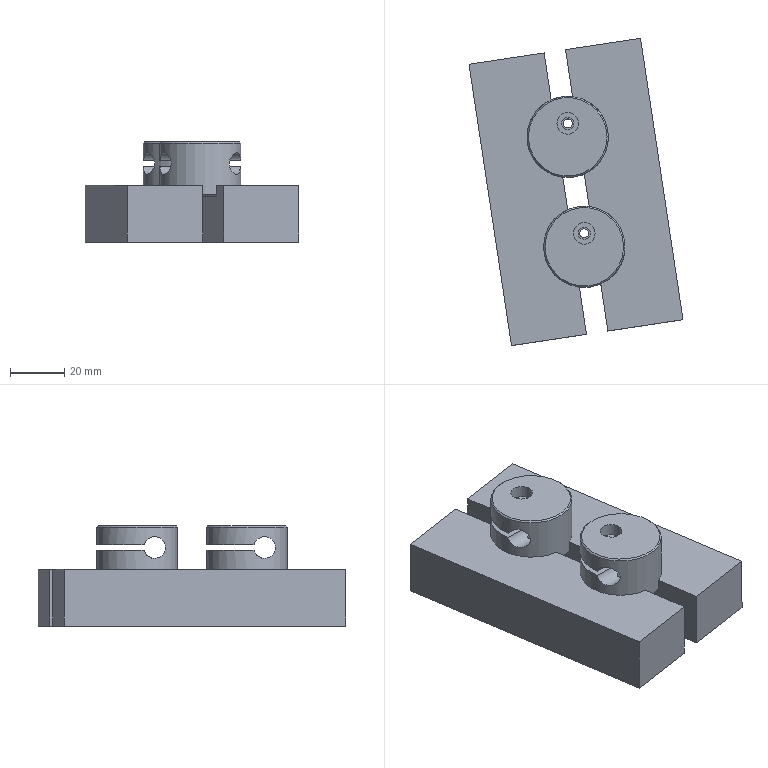CAM job | NX | 3-axis milling, drilling | part box 78.946 x 113.372 x 37 mm
Tools:
number,name,description,diameter,corner_radius,flute_length,length,flutes
3,D3,平底铣刀-粗,3.0,0.0,20.0,75.0,2
4,D4,平底铣刀-粗,4.0,0.0,25.0,75.0,2
8,D8,平底铣刀-粗,8.0,0.0,30.0,75.0,2
9,D10,平底铣刀-粗,10.0,0.0,35.0,75.0,2
10,D10-J,平底铣刀-精,10.0,0.0,35.0,75.0,2
1,D80R0.8飞刀,圆鼻刀-粗,80.0,0.8,50.0,75.0,2
2,D6倒角刀,倒角刀,6.0,0.0,3.0,25.0,2
20,M3X0.5,丝锥,2.5,0.0,35.0,50.0,2
21,M4X0.7,丝锥,3.3,0.0,35.0,50.0,2
12,ZT2.5,钻头,2.5,0.0,35.0,50.0,2
13,钻头3.3,Twist Drill 3.3 mm,3.3,0.0,35.0,35.008,2
Operations:
program,operation,operation_type,tool,method,geometry_group,spindle_rpm,surface_speed,feed_per_tooth,feed_cut,feed_plunge,cut_length_mm,path_length_mm,cut_time_min,machine_time_min
A,顶面,FaceMilling,D80R0.8飞刀,侧刃精光-切深K-步距G,W-A,4000.0,1005.31,0.125,1000.0,100.0,165.0,201.0,0.165,0.1686
A,动态开粗D8_COPY,CavityMilling,D8,动态开粗-切深K-步距K,W-A,8000.0,201.056,0.2188,3500.0,100.0,5250.862,5356.356,1.5,1.511
A,打点-深0.8,Operation,D6倒角刀,NONE,W-A,8000.0,150.796,0.0312,500.0,90.0,21.6,201.996,0.0432,0.0612
A,通孔-M3螺纹底孔,Operation,ZT2.5,NONE,W-A,3000.0,23.562,0.05,300.0,90.0,93.0,301.446,0.31,0.3308
A,盲锥孔-M3螺纹底孔,Operation,ZT2.5,NONE,W-A,3000.0,23.562,0.0167,100.0,90.0,64.0,234.601,0.64,0.6571
A,通孔-M4螺纹底孔,Operation,钻头3.3,NONE,W-A,3000.0,31.102,0.05,300.0,90.0,48.0,178.012,0.16,0.173
A,钻倒角_1,Operation,D6倒角刀,METHOD,W-A,8000.0,150.796,0.0312,500.0,0.0,47.5,272.832,0.095,0.1175
A,钻倒角_2,Operation,D6倒角刀,METHOD,W-A,8000.0,150.796,0.0312,500.0,0.0,10.4,104.91,0.0208,0.0303
A,底壁铣倒角_COPY,VolumeBased25DMillingOperation,D6倒角刀,爬面_倒角-切深0-步距G,W-A,6500.0,122.519,0.1154,1500.0,100.0,211.461,346.764,0.141,0.1545
A,盲锥孔-攻牙M3,Operation,M3X0.5,METHOD,W-A,1000.0,7.854,0.0003,0.5,90.0,48.0,202.601,96.0,96.016
A,通孔-攻牙M3,Operation,M3X0.5,METHOD,W-A,800.0,6.283,0.0003,0.5,90.0,78.0,271.446,156.0,156.019
A,通孔-攻牙M4,Operation,M4X0.7,METHOD,W-A,600.0,6.22,0.0006,0.7,90.0,30.0,142.012,42.857,42.868
A,外形半精_2,VolumeBased25DMillingOperation,D10-J,METHOD,W-A,8000.0,251.327,0.0625,1000.0,100.0,522.631,884.972,0.5226,0.5589
B,面铣自动飞面开粗一刀_COPY,FaceMilling,D80R0.8飞刀,分层开粗-切深K-步距G,W-B,4500.0,890.615,0.3333,3000.0,100.0,1917.474,3709.517,0.6392,0.8184
B,面铣自动飞面精光一刀_COPY,FaceMilling,D80R0.8飞刀,侧刃精光-切深K-步距G,W-B,4500.0,890.615,0.1111,1000.0,100.0,213.053,309.053,0.2131,0.2227
B,三段孔-铣孔开粗1_1,CylinderMilling,D4,NONE,W-B,8000.0,100.531,0.075,1200.0,100.0,453.457,702.657,0.3779,0.4028
B,三段孔-铣孔精光1_1,CylinderMilling,D4,精光步距切深关,W-B,8000.0,100.531,0.0312,500.0,100.0,65.174,314.374,0.1303,0.1553
B,三段孔-铣孔开粗2_1,CylinderMilling,D3,NONE,W-B,8000.0,100.531,0.075,1200.0,100.0,113.12,377.32,0.0943,0.1207
B,三段孔-铣孔精光2_1,CylinderMilling,D3,精光步距切深关,W-B,8000.0,100.531,0.0312,500.0,100.0,23.22,287.42,0.0464,0.0729
B,平面去毛刺6X45L_COPY,SurfaceContour,D6倒角刀,爬面_倒角-切深0-步距G,W-B,6500.0,122.519,0.1154,1500.0,100.0,566.809,950.273,0.3779,0.4162
B,底壁铣倒角_COPY_1,VolumeBased25DMillingOperation,D6倒角刀,爬面_倒角-切深0-步距G,W-B,6500.0,122.519,0.1154,1500.0,100.0,105.731,205.131,0.0705,0.0804
B,底壁铣倒角_COPY_2,VolumeBased25DMillingOperation,D6倒角刀,爬面_倒角-切深0-步距G,W-B,6500.0,122.519,0.1154,1500.0,100.0,105.731,205.131,0.0705,0.0804
C,底壁铣分层开粗-中_COPY,VolumeBased25DMillingOperation,D10,分层开粗-切深K-步距G,W-C,8000.0,251.32,0.25,4000.0,100.0,1874.82,2116.178,0.4687,0.4928
C,平面去毛刺6X45L_COPY_1,SurfaceContour,D6倒角刀,爬面_倒角-切深0-步距G,W-C,6500.0,122.519,0.1154,1500.0,100.0,161.213,442.357,0.1075,0.1356
C,平面铣精光侧面-中_COPY_1,PlanarMilling,D10-J,侧刃精光-切深K-步距G,W-C,8000.0,251.32,0.0625,1000.0,100.0,82.383,337.08,0.0824,0.1079
C,平面铣精光侧面-中_COPY_1_COPY,PlanarMilling,D10-J,侧刃精光-切深K-步距G,W-C,8000.0,251.32,0.0625,1000.0,100.0,144.298,398.432,0.1443,0.1697